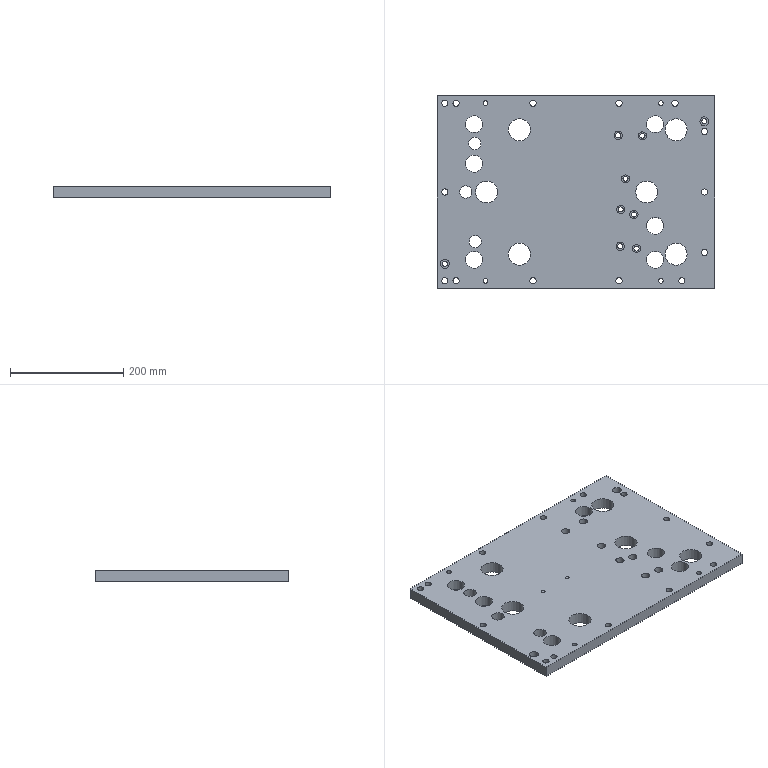Part | NX | features LIN_SOLID_COLOR 2 | 1 solid | 70 faces | box 490 x 340 x 20 mm | volume 3026473 mm3 | cylinder 53 | plane 17 | commonest cylinder face diameters 11 x14 9 x9 14.5 x7 30 x6 39 x6 8.5 x4